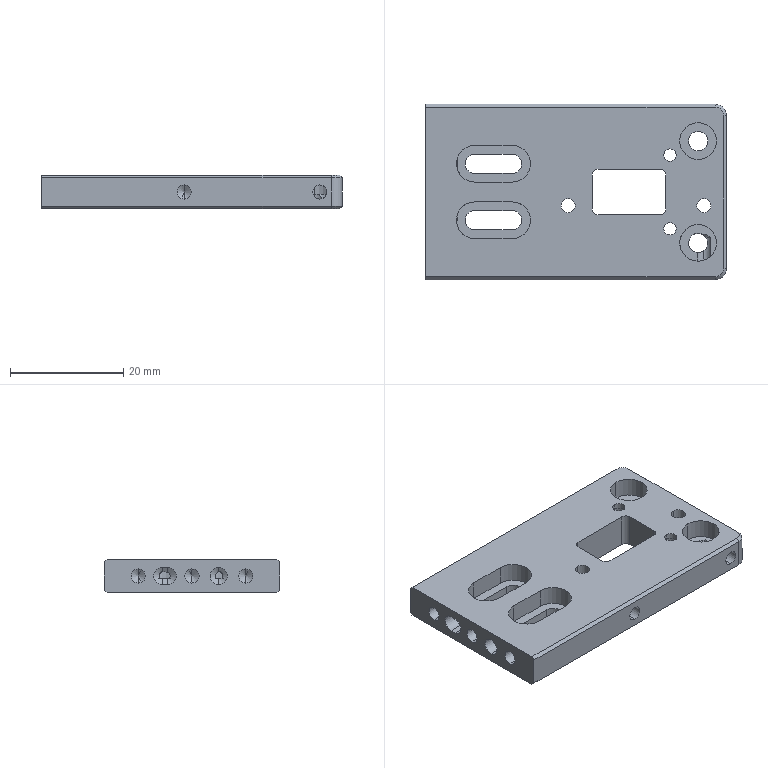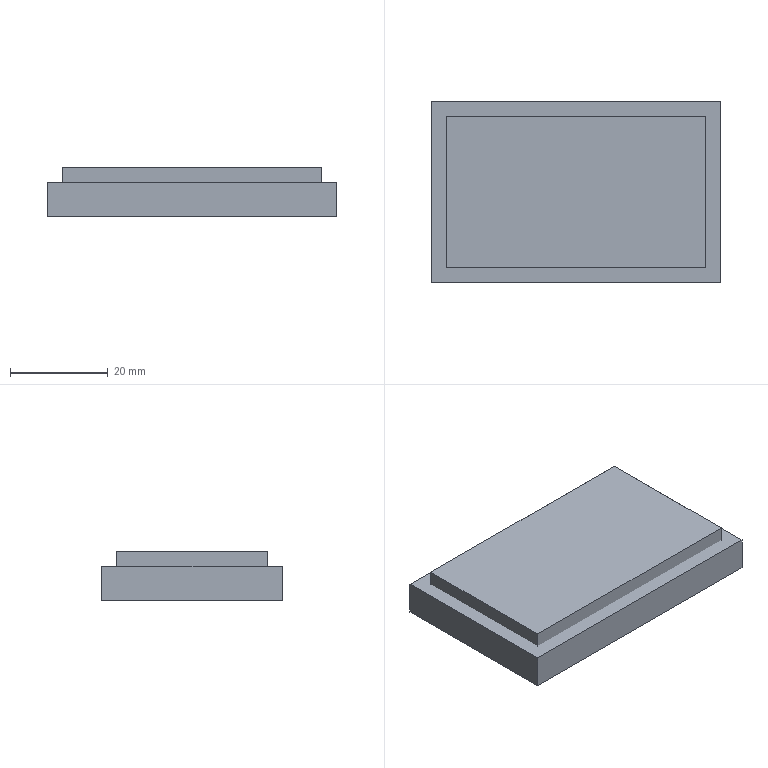CAM job | NX | 3+2 milling, drilling | part box 53.2 x 31 x 6 mm | stock box 59.2 x 37 x 10 mm
Tools:
number,name,description,diameter,corner_radius,flute_length,length,flutes
1,D50,Milling Tool-5 Parameters,50.0,0.0,50.0,75.0,2
7,D6A45,Milling Tool-5 Parameters,6.0,0.0,3.0,3.0,2
12,2.2ZT,Drilling Tool,2.2,0.0,35.0,50.0,2
13,3.4ZT,Drilling Tool,3.3,0.0,35.0,50.0,2
10,D10,Milling Tool-5 Parameters,10.0,0.0,50.0,75.0,2
6,D6,Milling Tool-5 Parameters,6.0,0.0,50.0,75.0,2
4,D4,Milling Tool-5 Parameters,4.0,0.0,50.0,75.0,2
2,D2,Milling Tool-5 Parameters,2.0,0.0,50.0,75.0,2
11,2.5ZT,Drilling Tool,2.5,0.0,35.0,50.0,2
Operations:
program,operation,operation_type,tool,method,geometry_group,spindle_rpm,surface_speed,feed_per_tooth,feed_cut,feed_plunge,cut_length_mm,path_length_mm,cut_time_min,machine_time_min
1-10-35-59毛胚,FLOOR_WALL,VolumeBased25DMillingOperation,D50,METHOD,A,6500.0,1286.0,0.0962,1250.0,100.0,121.2,175.2,0.097,0.1024
1-10-35-59毛胚,DRILLING_COPY_1,Operation,D6A45,METHOD,A,3000.0,56.0,0.0333,200.0,0.0,25.2,218.04,0.126,0.1453
1-10-35-59毛胚,DRILLING_COPY_1_COPY_COPY_COPY_COPY_COPY_COPY_COPY,Operation,2.2ZT,METHOD,A,2000.0,15.0,0.0375,150.0,0.0,21.322,118.986,0.1421,0.1519
1-10-35-59毛胚,DRILLING_COPY_1_COPY_COPY_COPY_COPY,Operation,3.4ZT,METHOD,A,2000.0,21.0,0.0375,150.0,0.0,20.983,123.214,0.1399,0.1501
1-10-35-59毛胚,DRILLING_COPY_1_COPY_COPY_COPY_COPY_COPY_COPY,Operation,2.5ZT,METHOD,A,2000.0,15.0,0.0375,150.0,0.0,20.502,128.191,0.1367,0.1474
1-10-35-59毛胚,ADAPTIVE_MILLING,CavityMilling,D10,METHOD,A,7000.0,219.0,0.2143,3000.0,1000.0,902.366,968.366,0.3028,0.3094
1-10-35-59毛胚,ZLEVEL_PROFILE_COPY,ZLevelMilling,D6,METHOD,A,7000.0,219.0,0.2143,3000.0,1000.0,308.791,371.791,0.1271,0.1334
1-10-35-59毛胚,ZLEVEL_PROFILE_COPY_1,ZLevelMilling,D4,METHOD,A,7000.0,87.0,0.1071,1500.0,1000.0,289.022,656.53,0.2149,0.2517
1-10-35-59毛胚,ZLEVEL_PROFILE_COPY_COPY,ZLevelMilling,D4,METHOD,A,7000.0,87.0,0.1,1400.0,1000.0,607.078,736.919,0.4531,0.4661
1-10-35-59毛胚,ZLEVEL_PROFILE_COPY_COPY_1_COPY_COPY_COPY_1,ZLevelMilling,D4,METHOD,A,7000.0,219.0,0.0714,1000.0,100.0,207.802,395.423,0.2078,0.2266
1-10-35-59毛胚,HOLE_MILLING,CylinderMilling,D4,METHOD,A,7000.0,131.0,0.1071,1500.0,100.0,227.914,371.714,0.1519,0.1663
1-10-35-59毛胚,ZLEVEL_PROFILE_COPY_COPY_COPY,ZLevelMilling,D2,METHOD,A,7000.0,65.0,0.0857,1200.0,1000.0,713.857,857.295,0.6054,0.6197
1-10-35-59毛胚,ZLEVEL_PROFILE_COPY_1_COPY_1,ZLevelMilling,D2,METHOD,A,7000.0,43.0,0.0786,1100.0,1000.0,444.285,927.448,0.41,0.4583
1-10-35-59毛胚,ZLEVEL_PROFILE_COPY_1_COPY_COPY_COPY_COPY_2_COPY_COPY_1,ZLevelMilling,D6A45,METHOD,A,7000.0,131.0,0.0714,1000.0,1000.0,314.744,992.35,0.3147,0.3825
2-10-35-59毛胚,FLOOR_WALL_COPY,VolumeBased25DMillingOperation,D50,METHOD,B,6500.0,1286.0,0.0962,1250.0,100.0,460.8,992.401,0.3686,0.4218
2-10-35-59毛胚,ZLEVEL_PROFILE_1,ZLevelMilling,D2,METHOD,B,7000.0,65.0,0.0786,1100.0,1000.0,240.06,378.784,0.2222,0.2361
2-10-35-59毛胚,ZLEVEL_PROFILE_COPY_1_COPY_COPY_COPY_COPY_2_COPY_COPY_1_1_COPY_1,ZLevelMilling,D6A45,METHOD,B,7000.0,131.0,0.0714,1000.0,1000.0,278.638,1096.022,0.2786,0.3604
2-10-35-59毛胚,刀补5.,ZLevelMilling,D2,METHOD,B,7000.0,65.0,0.0786,1100.0,1000.0,37.416,180.755,0.0342,0.0485
3-10-35-59毛胚,DRILLING_COPY_1_COPY_1,Operation,D6A45,METHOD,C,3000.0,56.0,0.0333,200.0,0.0,23.0,140.485,0.115,0.1267
3-10-35-59毛胚,DRILLING_COPY_1_COPY_COPY_COPY_COPY_COPY_COPY_1,Operation,2.5ZT,METHOD,C,2000.0,15.0,0.0375,150.0,0.0,51.165,219.748,0.3411,0.358
3-10-35-59毛胚,ZLEVEL_PROFILE_1_1,ZLevelMilling,D2,METHOD,C,7000.0,65.0,0.0786,1100.0,1000.0,309.534,444.555,0.2854,0.2989
3-10-35-59毛胚,ZLEVEL_PROFILE_COPY_1_COPY_COPY_COPY_COPY_2_COPY_COPY_1_1_COPY_1_1,ZLevelMilling,D6A45,METHOD,C,7000.0,131.0,0.0714,1000.0,1000.0,21.182,359.771,0.0212,0.055
3-10-35-59毛胚,刀补5._1,ZLevelMilling,D2,METHOD,C,7000.0,65.0,0.0786,1100.0,1000.0,48.64,188.225,0.0444,0.0583